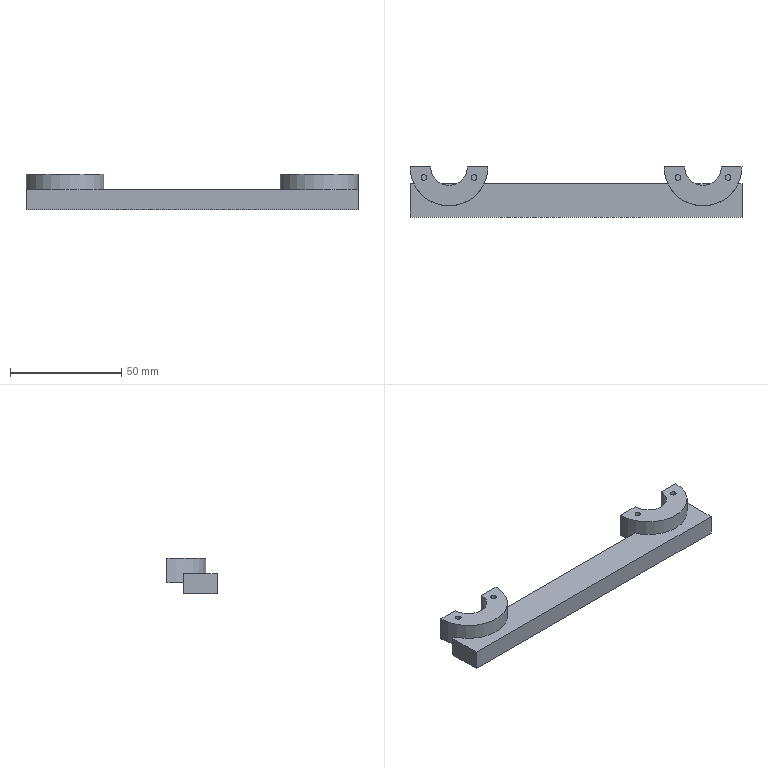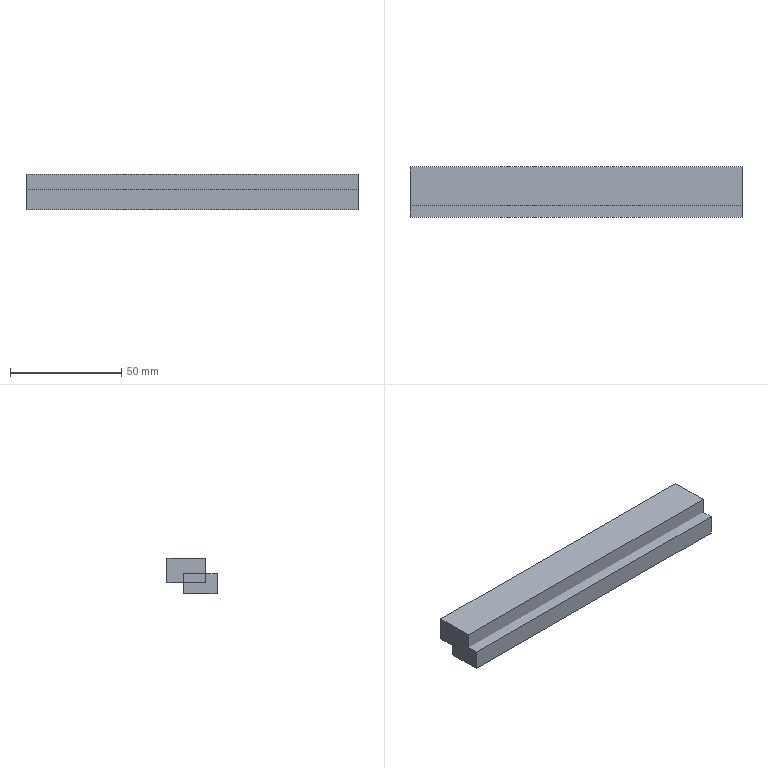CAM job | NX | 3-axis milling, drilling | part box 149 x 22.5 x 16 mm | stock box 149 x 22.5 x 16 mm
Tools:
number,name,description,diameter,corner_radius,flute_length,length,flutes
1,ZXZ,Milling Tool-5 Parameters,6.0,0.0,50.0,75.0,2
2,2.5ZT,Drilling Tool,2.5,0.0,35.0,50.0,2
2,D10,Milling Tool-5 Parameters,10.0,0.0,50.0,75.0,2
3,D6A45,Milling Tool-5 Parameters,6.0,0.0,50.0,75.0,2
Operations:
program,operation,operation_type,tool,method,geometry_group,spindle_rpm,surface_speed,feed_per_tooth,feed_cut,feed_plunge,cut_length_mm,path_length_mm,cut_time_min,machine_time_min
1,DRILLING,Operation,ZXZ,METHOD,A,3000.0,56.0,0.0333,200.0,0.0,16.0,237.947,0.08,0.1022
1,DRILLING_COPY,Operation,2.5ZT,METHOD,A,200.0,1.0,0.3,120.0,0.0,39.004,283.956,0.325,0.3495
1,DRILLING_COPY_1,Operation,D6A45,METHOD,A,3000.0,56.0,0.0333,200.0,0.0,17.6,241.147,0.088,0.1104
2,FLOOR_WALL,VolumeBased25DMillingOperation,D10,METHOD,B,9500.0,298.0,0.1316,2500.0,1000.0,475.137,771.819,0.2304,0.26
2,FLOOR_WALL_COPY,VolumeBased25DMillingOperation,D10,METHOD,B,9500.0,298.0,0.0526,1000.0,1000.0,231.6,492.544,0.2316,0.2577